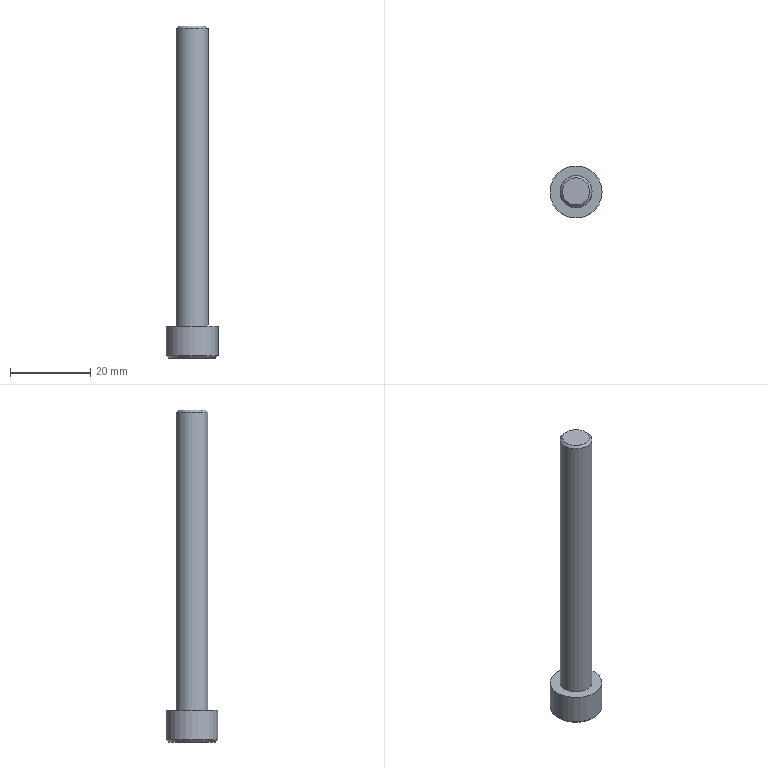Part | STEP file | M8.00-50.00 | 1 solid | 14 faces | box 13 x 13 x 83 mm | volume 4660 mm3 | plane 10 | cylinder 2 | cone 2 | commonest cylinder face diameters 8 x1 13 x1